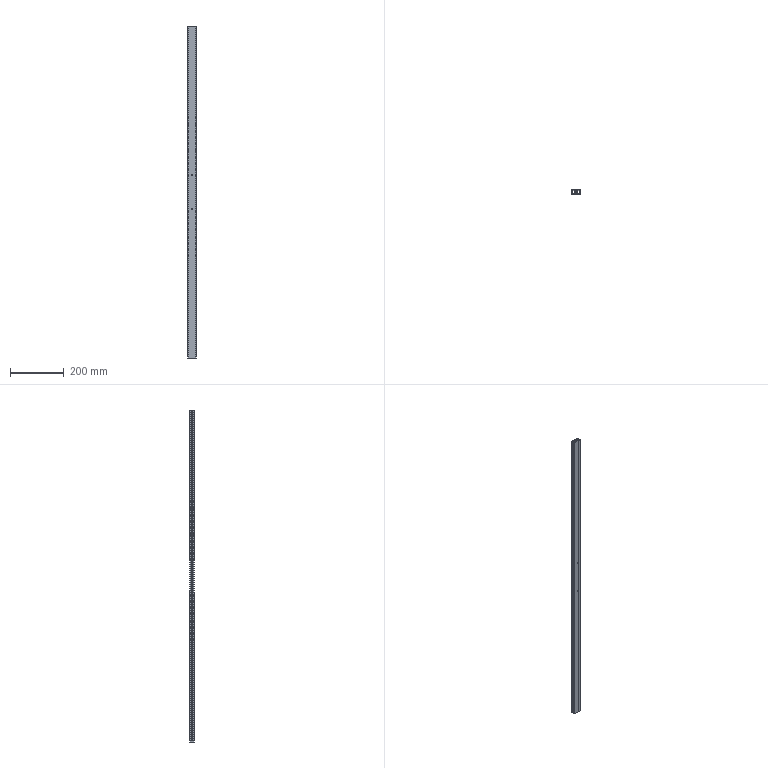Part | SolidWorks | features HoleWzd 3, BaseBody 1, MoveFace 1 | 1 solid | 160 faces | box 30 x 15 x 1236 mm | volume 297203 mm3 | cylinder 76 | plane 72 | cone 12 | commonest cylinder face diameters 5 x22 3.3 x16 4.5 x16 1 x12 2 x4 6.6 x4